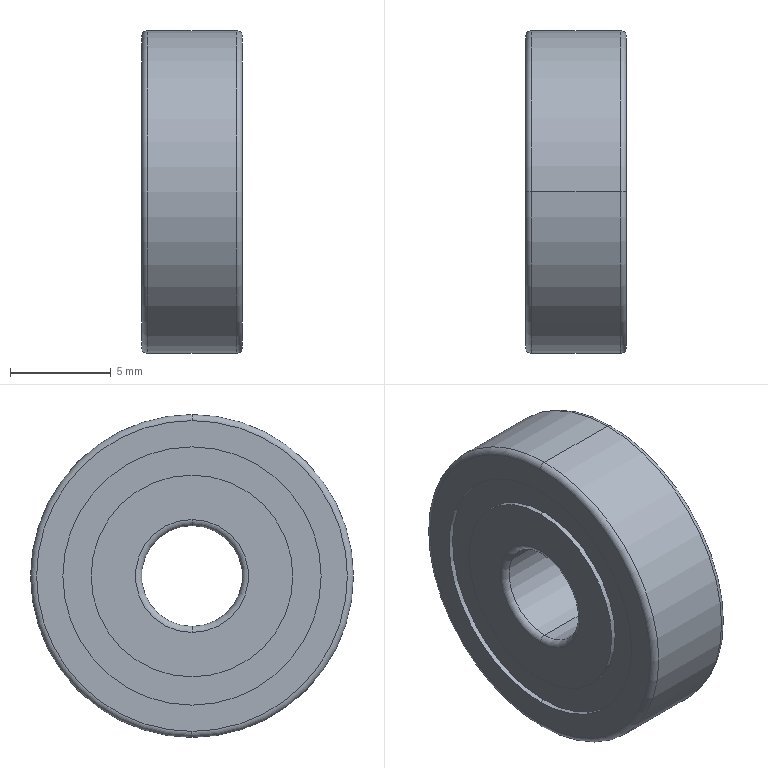Part | SolidWorks | features Revolution 1 | 1 solid | 26 faces | box 5 x 16 x 16 mm | volume 879.517 mm3 | cylinder 12 | torus 8 | plane 6 | commonest cylinder face diameters 10 x4 12.8 x4 5 x2 16 x2
STEP:
#1=CARTESIAN_POINT('',(2.2,0.,8.));
#2=VERTEX_POINT('',#1);
#3=CARTESIAN_POINT('',(2.2,0.,-8.));
#4=VERTEX_POINT('',#3);
#5=CARTESIAN_POINT('',(2.2,0.,0.));
#6=DIRECTION('',(-1.,0.,0.));
#7=DIRECTION('',(0.,0.,1.));
#8=AXIS2_PLACEMENT_3D('',#5,#6,#7);
#9=CIRCLE('',#8,8.);
#10=EDGE_CURVE('',#2,#4,#9,.T.);
#11=ORIENTED_EDGE('',*,*,#10,.T.);
#12=CARTESIAN_POINT('',(-2.2,0.,-8.));
#13=VERTEX_POINT('',#12);
#14=CARTESIAN_POINT('',(2.5,0.,-8.));
#15=DIRECTION('',(-1.,0.,0.));
#16=VECTOR('',#15,1000.);
#17=LINE('',#14,#16);
#18=EDGE_CURVE('',#4,#13,#17,.T.);
#19=ORIENTED_EDGE('',*,*,#18,.T.);
#20=CARTESIAN_POINT('',(-2.2,0.,8.));
#21=VERTEX_POINT('',#20);
#22=CARTESIAN_POINT('',(-2.2,0.,0.));
#23=DIRECTION('',(-1.,0.,0.));
#24=DIRECTION('',(0.,0.,1.));
#25=AXIS2_PLACEMENT_3D('',#22,#23,#24);
#26=CIRCLE('',#25,8.);
#27=EDGE_CURVE('',#21,#13,#26,.T.);
#28=ORIENTED_EDGE('',*,*,#27,.F.);
#29=CARTESIAN_POINT('',(2.5,0.,8.));
#30=DIRECTION('',(-1.,0.,0.));
#31=VECTOR('',#30,1000.);
#32=LINE('',#29,#31);
#33=EDGE_CURVE('',#2,#21,#32,.T.);
#34=ORIENTED_EDGE('',*,*,#33,.F.);
#35=EDGE_LOOP('',(#11,#19,#28,#34));
#36=FACE_OUTER_BOUND('',#35,.T.);
#37=CARTESIAN_POINT('',(2.5,0.,0.));
#38=DIRECTION('',(-1.,0.,0.));
#39=DIRECTION('',(0.,0.,1.));
#40=AXIS2_PLACEMENT_3D('',#37,#38,#39);
#41=CYLINDRICAL_SURFACE('',#40,8.);
#42=ADVANCED_FACE('',(#36),#41,.T.);
#43=CARTESIAN_POINT('',(2.5,0.,7.7));
#44=VERTEX_POINT('',#43);
#45=CARTESIAN_POINT('',(2.5,0.,-7.7));
#46=VERTEX_POINT('',#45);
#47=CARTESIAN_POINT('',(2.5,0.,0.));
#48=DIRECTION('',(-1.,0.,0.));
#49=DIRECTION('',(0.,0.,1.));
#50=AXIS2_PLACEMENT_3D('',#47,#48,#49);
#51=CIRCLE('',#50,7.7);
#52=EDGE_CURVE('',#44,#46,#51,.T.);
#53=ORIENTED_EDGE('',*,*,#52,.T.);
#54=CARTESIAN_POINT('',(2.2,0.,-7.7));
#55=DIRECTION('',(0.,1.,0.));
#56=DIRECTION('',(0.,0.,1.));
#57=AXIS2_PLACEMENT_3D('',#54,#55,#56);
#58=CIRCLE('',#57,0.3);
#59=EDGE_CURVE('',#46,#4,#58,.T.);
#60=ORIENTED_EDGE('',*,*,#59,.T.);
#61=ORIENTED_EDGE('',*,*,#10,.F.);
#62=CARTESIAN_POINT('',(2.2,0.,7.7));
#63=DIRECTION('',(0.,-1.,0.));
#64=DIRECTION('',(0.,0.,-1.));
#65=AXIS2_PLACEMENT_3D('',#62,#63,#64);
#66=CIRCLE('',#65,0.3);
#67=EDGE_CURVE('',#44,#2,#66,.T.);
#68=ORIENTED_EDGE('',*,*,#67,.F.);
#69=EDGE_LOOP('',(#53,#60,#61,#68));
#70=FACE_OUTER_BOUND('',#69,.T.);
#71=CARTESIAN_POINT('',(2.2,0.,0.));
#72=DIRECTION('',(-1.,0.,0.));
#73=DIRECTION('',(0.,0.,1.));
#74=AXIS2_PLACEMENT_3D('',#71,#72,#73);
#75=TOROIDAL_SURFACE('',#74,7.7,0.3);
#76=ADVANCED_FACE('',(#70),#75,.T.);
#77=CARTESIAN_POINT('',(2.5,0.,-6.4));
#78=VERTEX_POINT('',#77);
#79=CARTESIAN_POINT('',(2.5,0.,6.4));
#80=VERTEX_POINT('',#79);
#81=CARTESIAN_POINT('',(2.5,0.,0.));
#82=DIRECTION('',(-1.,0.,0.));
#83=DIRECTION('',(0.,0.,1.));
#84=AXIS2_PLACEMENT_3D('',#81,#82,#83);
#85=CIRCLE('',#84,6.4);
#86=EDGE_CURVE('',#78,#80,#85,.T.);
#87=ORIENTED_EDGE('',*,*,#86,.F.);
#88=CARTESIAN_POINT('',(2.25,0.,-6.4));
#89=VERTEX_POINT('',#88);
#90=CARTESIAN_POINT('',(2.5,0.,-6.4));
#91=DIRECTION('',(-1.,0.,0.));
#92=VECTOR('',#91,1000.);
#93=LINE('',#90,#92);
#94=EDGE_CURVE('',#78,#89,#93,.T.);
#95=ORIENTED_EDGE('',*,*,#94,.T.);
#96=CARTESIAN_POINT('',(2.25,0.,6.4));
#97=VERTEX_POINT('',#96);
#98=CARTESIAN_POINT('',(2.25,0.,0.));
#99=DIRECTION('',(-1.,0.,0.));
#100=DIRECTION('',(0.,0.,1.));
#101=AXIS2_PLACEMENT_3D('',#98,#99,#100);
#102=CIRCLE('',#101,6.4);
#103=EDGE_CURVE('',#89,#97,#102,.T.);
#104=ORIENTED_EDGE('',*,*,#103,.T.);
#105=CARTESIAN_POINT('',(2.5,0.,6.4));
#106=DIRECTION('',(-1.,0.,0.));
#107=VECTOR('',#106,1000.);
#108=LINE('',#105,#107);
#109=EDGE_CURVE('',#80,#97,#108,.T.);
#110=ORIENTED_EDGE('',*,*,#109,.F.);
#111=EDGE_LOOP('',(#87,#95,#104,#110));
#112=FACE_OUTER_BOUND('',#111,.T.);
#113=CARTESIAN_POINT('',(2.5,0.,0.));
#114=DIRECTION('',(-1.,0.,0.));
#115=DIRECTION('',(0.,0.,1.));
#116=AXIS2_PLACEMENT_3D('',#113,#114,#115);
#117=CYLINDRICAL_SURFACE('',#116,6.4);
#118=ADVANCED_FACE('',(#112),#117,.F.);
#119=CARTESIAN_POINT('',(2.5,0.,5.));
#120=VERTEX_POINT('',#119);
#121=CARTESIAN_POINT('',(2.5,0.,-5.));
#122=VERTEX_POINT('',#121);
#123=CARTESIAN_POINT('',(2.5,0.,0.));
#124=DIRECTION('',(-1.,0.,0.));
#125=DIRECTION('',(0.,0.,1.));
#126=AXIS2_PLACEMENT_3D('',#123,#124,#125);
#127=CIRCLE('',#126,5.);
#128=EDGE_CURVE('',#120,#122,#127,.T.);
#129=ORIENTED_EDGE('',*,*,#128,.T.);
#130=CARTESIAN_POINT('',(2.25,0.,-5.));
#131=VERTEX_POINT('',#130);
#132=CARTESIAN_POINT('',(2.5,0.,-5.));
#133=DIRECTION('',(-1.,0.,0.));
#134=VECTOR('',#133,1000.);
#135=LINE('',#132,#134);
#136=EDGE_CURVE('',#122,#131,#135,.T.);
#137=ORIENTED_EDGE('',*,*,#136,.T.);
#138=CARTESIAN_POINT('',(2.25,0.,5.));
#139=VERTEX_POINT('',#138);
#140=CARTESIAN_POINT('',(2.25,0.,0.));
#141=DIRECTION('',(-1.,0.,0.));
#142=DIRECTION('',(0.,0.,1.));
#143=AXIS2_PLACEMENT_3D('',#140,#141,#142);
#144=CIRCLE('',#143,5.);
#145=EDGE_CURVE('',#139,#131,#144,.T.);
#146=ORIENTED_EDGE('',*,*,#145,.F.);
#147=CARTESIAN_POINT('',(2.5,0.,5.));
#148=DIRECTION('',(-1.,0.,0.));
#149=VECTOR('',#148,1000.);
#150=LINE('',#147,#149);
#151=EDGE_CURVE('',#120,#139,#150,.T.);
#152=ORIENTED_EDGE('',*,*,#151,.F.);
#153=EDGE_LOOP('',(#129,#137,#146,#152));
#154=FACE_OUTER_BOUND('',#153,.T.);
#155=CARTESIAN_POINT('',(2.5,0.,0.));
#156=DIRECTION('',(-1.,0.,0.));
#157=DIRECTION('',(0.,0.,1.));
#158=AXIS2_PLACEMENT_3D('',#155,#156,#157);
#159=CYLINDRICAL_SURFACE('',#158,5.);
#160=ADVANCED_FACE('',(#154),#159,.T.);
#161=CARTESIAN_POINT('',(2.2,0.,2.5));
#162=VERTEX_POINT('',#161);
#163=CARTESIAN_POINT('',(2.2,0.,-2.5));
#164=VERTEX_POINT('',#163);
#165=CARTESIAN_POINT('',(2.2,0.,0.));
#166=DIRECTION('',(-1.,0.,0.));
#167=DIRECTION('',(0.,0.,1.));
#168=AXIS2_PLACEMENT_3D('',#165,#166,#167);
#169=CIRCLE('',#168,2.5);
#170=EDGE_CURVE('',#162,#164,#169,.T.);
#171=ORIENTED_EDGE('',*,*,#170,.T.);
#172=CARTESIAN_POINT('',(2.5,0.,-2.8));
#173=VERTEX_POINT('',#172);
#174=CARTESIAN_POINT('',(2.2,0.,-2.8));
#175=DIRECTION('',(0.,1.,0.));
#176=DIRECTION('',(0.,0.,1.));
#177=AXIS2_PLACEMENT_3D('',#174,#175,#176);
#178=CIRCLE('',#177,0.3);
#179=EDGE_CURVE('',#164,#173,#178,.T.);
#180=ORIENTED_EDGE('',*,*,#179,.T.);
#181=CARTESIAN_POINT('',(2.5,0.,2.8));
#182=VERTEX_POINT('',#181);
#183=CARTESIAN_POINT('',(2.5,0.,0.));
#184=DIRECTION('',(-1.,0.,0.));
#185=DIRECTION('',(0.,0.,1.));
#186=AXIS2_PLACEMENT_3D('',#183,#184,#185);
#187=CIRCLE('',#186,2.8);
#188=EDGE_CURVE('',#182,#173,#187,.T.);
#189=ORIENTED_EDGE('',*,*,#188,.F.);
#190=CARTESIAN_POINT('',(2.2,0.,2.8));
#191=DIRECTION('',(0.,-1.,0.));
#192=DIRECTION('',(0.,0.,-1.));
#193=AXIS2_PLACEMENT_3D('',#190,#191,#192);
#194=CIRCLE('',#193,0.3);
#195=EDGE_CURVE('',#162,#182,#194,.T.);
#196=ORIENTED_EDGE('',*,*,#195,.F.);
#197=EDGE_LOOP('',(#171,#180,#189,#196));
#198=FACE_OUTER_BOUND('',#197,.T.);
#199=CARTESIAN_POINT('',(2.2,0.,0.));
#200=DIRECTION('',(-1.,0.,0.));
#201=DIRECTION('',(0.,0.,1.));
#202=AXIS2_PLACEMENT_3D('',#199,#200,#201);
#203=TOROIDAL_SURFACE('',#202,2.8,0.3);
#204=ADVANCED_FACE('',(#198),#203,.T.);
#205=CARTESIAN_POINT('',(2.2,0.,0.));
#206=DIRECTION('',(-1.,0.,0.));
#207=DIRECTION('',(0.,0.,1.));
#208=AXIS2_PLACEMENT_3D('',#205,#206,#207);
#209=CIRCLE('',#208,2.5);
#210=EDGE_CURVE('',#164,#162,#209,.T.);
#211=ORIENTED_EDGE('',*,*,#210,.F.);
#212=CARTESIAN_POINT('',(-2.2,0.,-2.5));
#213=VERTEX_POINT('',#212);
#214=CARTESIAN_POINT('',(2.5,0.,-2.5));
#215=DIRECTION('',(-1.,0.,0.));
#216=VECTOR('',#215,1000.);
#217=LINE('',#214,#216);
#218=EDGE_CURVE('',#164,#213,#217,.T.);
#219=ORIENTED_EDGE('',*,*,#218,.T.);
#220=CARTESIAN_POINT('',(-2.2,0.,2.5));
#221=VERTEX_POINT('',#220);
#222=CARTESIAN_POINT('',(-2.2,0.,0.));
#223=DIRECTION('',(-1.,0.,0.));
#224=DIRECTION('',(0.,0.,1.));
#225=AXIS2_PLACEMENT_3D('',#222,#223,#224);
#226=CIRCLE('',#225,2.5);
#227=EDGE_CURVE('',#213,#221,#226,.T.);
#228=ORIENTED_EDGE('',*,*,#227,.T.);
#229=CARTESIAN_POINT('',(2.5,0.,2.5));
#230=DIRECTION('',(-1.,0.,0.));
#231=VECTOR('',#230,1000.);
#232=LINE('',#229,#231);
#233=EDGE_CURVE('',#162,#221,#232,.T.);
#234=ORIENTED_EDGE('',*,*,#233,.F.);
#235=EDGE_LOOP('',(#211,#219,#228,#234));
#236=FACE_OUTER_BOUND('',#235,.T.);
#237=CARTESIAN_POINT('',(2.5,0.,0.));
#238=DIRECTION('',(-1.,0.,0.));
#239=DIRECTION('',(0.,0.,1.));
#240=AXIS2_PLACEMENT_3D('',#237,#238,#239);
#241=CYLINDRICAL_SURFACE('',#240,2.5);
#242=ADVANCED_FACE('',(#236),#241,.F.);
#243=CARTESIAN_POINT('',(-2.5,0.,2.8));
#244=VERTEX_POINT('',#243);
#245=CARTESIAN_POINT('',(-2.5,0.,-2.8));
#246=VERTEX_POINT('',#245);
#247=CARTESIAN_POINT('',(-2.5,0.,0.));
#248=DIRECTION('',(-1.,0.,0.));
#249=DIRECTION('',(0.,0.,1.));
#250=AXIS2_PLACEMENT_3D('',#247,#248,#249);
#251=CIRCLE('',#250,2.8);
#252=EDGE_CURVE('',#244,#246,#251,.T.);
#253=ORIENTED_EDGE('',*,*,#252,.T.);
#254=CARTESIAN_POINT('',(-2.2,0.,-2.8));
#255=DIRECTION('',(0.,1.,0.));
#256=DIRECTION('',(0.,0.,1.));
#257=AXIS2_PLACEMENT_3D('',#254,#255,#256);
#258=CIRCLE('',#257,0.3);
#259=EDGE_CURVE('',#246,#213,#258,.T.);
#260=ORIENTED_EDGE('',*,*,#259,.T.);
#261=CARTESIAN_POINT('',(-2.2,0.,0.));
#262=DIRECTION('',(-1.,0.,0.));
#263=DIRECTION('',(0.,0.,1.));
#264=AXIS2_PLACEMENT_3D('',#261,#262,#263);
#265=CIRCLE('',#264,2.5);
#266=EDGE_CURVE('',#221,#213,#265,.T.);
#267=ORIENTED_EDGE('',*,*,#266,.F.);
#268=CARTESIAN_POINT('',(-2.2,0.,2.8));
#269=DIRECTION('',(0.,-1.,0.));
#270=DIRECTION('',(0.,0.,-1.));
#271=AXIS2_PLACEMENT_3D('',#268,#269,#270);
#272=CIRCLE('',#271,0.3);
#273=EDGE_CURVE('',#244,#221,#272,.T.);
#274=ORIENTED_EDGE('',*,*,#273,.F.);
#275=EDGE_LOOP('',(#253,#260,#267,#274));
#276=FACE_OUTER_BOUND('',#275,.T.);
#277=CARTESIAN_POINT('',(-2.2,0.,0.));
#278=DIRECTION('',(-1.,0.,0.));
#279=DIRECTION('',(0.,0.,1.));
#280=AXIS2_PLACEMENT_3D('',#277,#278,#279);
#281=TOROIDAL_SURFACE('',#280,2.8,0.3);
#282=ADVANCED_FACE('',(#276),#281,.T.);
#283=CARTESIAN_POINT('',(-2.25,0.,5.));
#284=VERTEX_POINT('',#283);
#285=CARTESIAN_POINT('',(-2.25,0.,-5.));
#286=VERTEX_POINT('',#285);
#287=CARTESIAN_POINT('',(-2.25,0.,0.));
#288=DIRECTION('',(-1.,0.,0.));
#289=DIRECTION('',(0.,0.,1.));
#290=AXIS2_PLACEMENT_3D('',#287,#288,#289);
#291=CIRCLE('',#290,5.);
#292=EDGE_CURVE('',#284,#286,#291,.T.);
#293=ORIENTED_EDGE('',*,*,#292,.T.);
#294=CARTESIAN_POINT('',(-2.5,0.,-5.));
#295=VERTEX_POINT('',#294);
#296=CARTESIAN_POINT('',(2.5,0.,-5.));
#297=DIRECTION('',(-1.,0.,0.));
#298=VECTOR('',#297,1000.);
#299=LINE('',#296,#298);
#300=EDGE_CURVE('',#286,#295,#299,.T.);
#301=ORIENTED_EDGE('',*,*,#300,.T.);
#302=CARTESIAN_POINT('',(-2.5,0.,5.));
#303=VERTEX_POINT('',#302);
#304=CARTESIAN_POINT('',(-2.5,0.,0.));
#305=DIRECTION('',(-1.,0.,0.));
#306=DIRECTION('',(0.,0.,1.));
#307=AXIS2_PLACEMENT_3D('',#304,#305,#306);
#308=CIRCLE('',#307,5.);
#309=EDGE_CURVE('',#303,#295,#308,.T.);
#310=ORIENTED_EDGE('',*,*,#309,.F.);
#311=CARTESIAN_POINT('',(2.5,0.,5.));
#312=DIRECTION('',(-1.,0.,0.));
#313=VECTOR('',#312,1000.);
#314=LINE('',#311,#313);
#315=EDGE_CURVE('',#284,#303,#314,.T.);
#316=ORIENTED_EDGE('',*,*,#315,.F.);
#317=EDGE_LOOP('',(#293,#301,#310,#316));
#318=FACE_OUTER_BOUND('',#317,.T.);
#319=CARTESIAN_POINT('',(2.5,0.,0.));
#320=DIRECTION('',(-1.,0.,0.));
#321=DIRECTION('',(0.,0.,1.));
#322=AXIS2_PLACEMENT_3D('',#319,#320,#321);
#323=CYLINDRICAL_SURFACE('',#322,5.);
#324=ADVANCED_FACE('',(#318),#323,.T.);
#325=CARTESIAN_POINT('',(-2.25,0.,-6.4));
#326=VERTEX_POINT('',#325);
#327=CARTESIAN_POINT('',(-2.25,0.,6.4));
#328=VERTEX_POINT('',#327);
#329=CARTESIAN_POINT('',(-2.25,0.,0.));
#330=DIRECTION('',(-1.,0.,0.));
#331=DIRECTION('',(0.,0.,1.));
#332=AXIS2_PLACEMENT_3D('',#329,#330,#331);
#333=CIRCLE('',#332,6.4);
#334=EDGE_CURVE('',#326,#328,#333,.T.);
#335=ORIENTED_EDGE('',*,*,#334,.F.);
#336=CARTESIAN_POINT('',(-2.5,0.,-6.4));
#337=VERTEX_POINT('',#336);
#338=CARTESIAN_POINT('',(2.5,0.,-6.4));
#339=DIRECTION('',(-1.,0.,0.));
#340=VECTOR('',#339,1000.);
#341=LINE('',#338,#340);
#342=EDGE_CURVE('',#326,#337,#341,.T.);
#343=ORIENTED_EDGE('',*,*,#342,.T.);
#344=CARTESIAN_POINT('',(-2.5,0.,6.4));
#345=VERTEX_POINT('',#344);
#346=CARTESIAN_POINT('',(-2.5,0.,0.));
#347=DIRECTION('',(-1.,0.,0.));
#348=DIRECTION('',(0.,0.,1.));
#349=AXIS2_PLACEMENT_3D('',#346,#347,#348);
#350=CIRCLE('',#349,6.4);
#351=EDGE_CURVE('',#337,#345,#350,.T.);
#352=ORIENTED_EDGE('',*,*,#351,.T.);
#353=CARTESIAN_POINT('',(2.5,0.,6.4));
#354=DIRECTION('',(-1.,0.,0.));
#355=VECTOR('',#354,1000.);
#356=LINE('',#353,#355);
#357=EDGE_CURVE('',#328,#345,#356,.T.);
#358=ORIENTED_EDGE('',*,*,#357,.F.);
#359=EDGE_LOOP('',(#335,#343,#352,#358));
#360=FACE_OUTER_BOUND('',#359,.T.);
#361=CARTESIAN_POINT('',(2.5,0.,0.));
#362=DIRECTION('',(-1.,0.,0.));
#363=DIRECTION('',(0.,0.,1.));
#364=AXIS2_PLACEMENT_3D('',#361,#362,#363);
#365=CYLINDRICAL_SURFACE('',#364,6.4);
#366=ADVANCED_FACE('',(#360),#365,.F.);
#367=ORIENTED_EDGE('',*,*,#27,.T.);
#368=CARTESIAN_POINT('',(-2.5,0.,-7.7));
#369=VERTEX_POINT('',#368);
#370=CARTESIAN_POINT('',(-2.2,0.,-7.7));
#371=DIRECTION('',(0.,1.,0.));
#372=DIRECTION('',(0.,0.,1.));
#373=AXIS2_PLACEMENT_3D('',#370,#371,#372);
#374=CIRCLE('',#373,0.3);
#375=EDGE_CURVE('',#13,#369,#374,.T.);
#376=ORIENTED_EDGE('',*,*,#375,.T.);
#377=CARTESIAN_POINT('',(-2.5,0.,7.7));
#378=VERTEX_POINT('',#377);
#379=CARTESIAN_POINT('',(-2.5,0.,0.));
#380=DIRECTION('',(-1.,0.,0.));
#381=DIRECTION('',(0.,0.,1.));
#382=AXIS2_PLACEMENT_3D('',#379,#380,#381);
#383=CIRCLE('',#382,7.7);
#384=EDGE_CURVE('',#378,#369,#383,.T.);
#385=ORIENTED_EDGE('',*,*,#384,.F.);
#386=CARTESIAN_POINT('',(-2.2,0.,7.7));
#387=DIRECTION('',(0.,-1.,0.));
#388=DIRECTION('',(0.,0.,-1.));
#389=AXIS2_PLACEMENT_3D('',#386,#387,#388);
#390=CIRCLE('',#389,0.3);
#391=EDGE_CURVE('',#21,#378,#390,.T.);
#392=ORIENTED_EDGE('',*,*,#391,.F.);
#393=EDGE_LOOP('',(#367,#376,#385,#392));
#394=FACE_OUTER_BOUND('',#393,.T.);
#395=CARTESIAN_POINT('',(-2.2,0.,0.));
#396=DIRECTION('',(-1.,0.,0.));
#397=DIRECTION('',(0.,0.,1.));
#398=AXIS2_PLACEMENT_3D('',#395,#396,#397);
#399=TOROIDAL_SURFACE('',#398,7.7,0.3);
#400=ADVANCED_FACE('',(#394),#399,.T.);
#401=ORIENTED_EDGE('',*,*,#375,.F.);
#402=CARTESIAN_POINT('',(-2.2,0.,0.));
#403=DIRECTION('',(-1.,0.,0.));
#404=DIRECTION('',(0.,0.,1.));
#405=AXIS2_PLACEMENT_3D('',#402,#403,#404);
#406=CIRCLE('',#405,8.);
#407=EDGE_CURVE('',#13,#21,#406,.T.);
#408=ORIENTED_EDGE('',*,*,#407,.T.);
#409=ORIENTED_EDGE('',*,*,#391,.T.);
#410=CARTESIAN_POINT('',(-2.5,0.,0.));
#411=DIRECTION('',(-1.,0.,0.));
#412=DIRECTION('',(0.,0.,1.));
#413=AXIS2_PLACEMENT_3D('',#410,#411,#412);
#414=CIRCLE('',#413,7.7);
#415=EDGE_CURVE('',#369,#378,#414,.T.);
#416=ORIENTED_EDGE('',*,*,#415,.F.);
#417=EDGE_LOOP('',(#401,#408,#409,#416));
#418=FACE_OUTER_BOUND('',#417,.T.);
#419=CARTESIAN_POINT('',(-2.2,0.,0.));
#420=DIRECTION('',(-1.,0.,0.));
#421=DIRECTION('',(0.,0.,1.));
#422=AXIS2_PLACEMENT_3D('',#419,#420,#421);
#423=TOROIDAL_SURFACE('',#422,7.7,0.3);
#424=ADVANCED_FACE('',(#418),#423,.T.);
#425=CARTESIAN_POINT('',(-2.5,0.,0.));
#426=DIRECTION('',(-1.,0.,0.));
#427=DIRECTION('',(0.,0.,1.));
#428=AXIS2_PLACEMENT_3D('',#425,#426,#427);
#429=CIRCLE('',#428,6.4);
#430=EDGE_CURVE('',#345,#337,#429,.T.);
#431=ORIENTED_EDGE('',*,*,#430,.F.);
#432=ORIENTED_EDGE('',*,*,#351,.F.);
#433=EDGE_LOOP('',(#431,#432));
#434=FACE_BOUND('',#433,.T.);
#435=ORIENTED_EDGE('',*,*,#384,.T.);
#436=ORIENTED_EDGE('',*,*,#415,.T.);
#437=EDGE_LOOP('',(#435,#436));
#438=FACE_OUTER_BOUND('',#437,.T.);
#439=CARTESIAN_POINT('',(-2.5,7.7,0.));
#440=DIRECTION('',(1.,0.,0.));
#441=DIRECTION('',(0.,0.,-1.));
#442=AXIS2_PLACEMENT_3D('',#439,#440,#441);
#443=PLANE('',#442);
#444=ADVANCED_FACE('',(#434,#438),#443,.F.);
#445=ORIENTED_EDGE('',*,*,#342,.F.);
#446=CARTESIAN_POINT('',(-2.25,0.,0.));
#447=DIRECTION('',(-1.,0.,0.));
#448=DIRECTION('',(0.,0.,1.));
#449=AXIS2_PLACEMENT_3D('',#446,#447,#448);
#450=CIRCLE('',#449,6.4);
#451=EDGE_CURVE('',#328,#326,#450,.T.);
#452=ORIENTED_EDGE('',*,*,#451,.F.);
#453=ORIENTED_EDGE('',*,*,#357,.T.);
#454=ORIENTED_EDGE('',*,*,#430,.T.);
#455=EDGE_LOOP('',(#445,#452,#453,#454));
#456=FACE_OUTER_BOUND('',#455,.T.);
#457=CARTESIAN_POINT('',(2.5,0.,0.));
#458=DIRECTION('',(-1.,0.,0.));
#459=DIRECTION('',(0.,0.,1.));
#460=AXIS2_PLACEMENT_3D('',#457,#458,#459);
#461=CYLINDRICAL_SURFACE('',#460,6.4);
#462=ADVANCED_FACE('',(#456),#461,.F.);
#463=ORIENTED_EDGE('',*,*,#292,.F.);
#464=CARTESIAN_POINT('',(-2.25,0.,0.));
#465=DIRECTION('',(-1.,0.,0.));
#466=DIRECTION('',(0.,0.,1.));
#467=AXIS2_PLACEMENT_3D('',#464,#465,#466);
#468=CIRCLE('',#467,5.);
#469=EDGE_CURVE('',#286,#284,#468,.T.);
#470=ORIENTED_EDGE('',*,*,#469,.F.);
#471=EDGE_LOOP('',(#463,#470));
#472=FACE_BOUND('',#471,.T.);
#473=ORIENTED_EDGE('',*,*,#451,.T.);
#474=ORIENTED_EDGE('',*,*,#334,.T.);
#475=EDGE_LOOP('',(#473,#474));
#476=FACE_OUTER_BOUND('',#475,.T.);
#477=CARTESIAN_POINT('',(-2.25,6.4,0.));
#478=DIRECTION('',(1.,0.,0.));
#479=DIRECTION('',(0.,0.,-1.));
#480=AXIS2_PLACEMENT_3D('',#477,#478,#479);
#481=PLANE('',#480);
#482=ADVANCED_FACE('',(#472,#476),#481,.F.);
#483=ORIENTED_EDGE('',*,*,#300,.F.);
#484=ORIENTED_EDGE('',*,*,#469,.T.);
#485=ORIENTED_EDGE('',*,*,#315,.T.);
#486=CARTESIAN_POINT('',(-2.5,0.,0.));
#487=DIRECTION('',(-1.,0.,0.));
#488=DIRECTION('',(0.,0.,1.));
#489=AXIS2_PLACEMENT_3D('',#486,#487,#488);
#490=CIRCLE('',#489,5.);
#491=EDGE_CURVE('',#295,#303,#490,.T.);
#492=ORIENTED_EDGE('',*,*,#491,.F.);
#493=EDGE_LOOP('',(#483,#484,#485,#492));
#494=FACE_OUTER_BOUND('',#493,.T.);
#495=CARTESIAN_POINT('',(2.5,0.,0.));
#496=DIRECTION('',(-1.,0.,0.));
#497=DIRECTION('',(0.,0.,1.));
#498=AXIS2_PLACEMENT_3D('',#495,#496,#497);
#499=CYLINDRICAL_SURFACE('',#498,5.);
#500=ADVANCED_FACE('',(#494),#499,.T.);
#501=ORIENTED_EDGE('',*,*,#252,.F.);
#502=CARTESIAN_POINT('',(-2.5,0.,0.));
#503=DIRECTION('',(-1.,0.,0.));
#504=DIRECTION('',(0.,0.,1.));
#505=AXIS2_PLACEMENT_3D('',#502,#503,#504);
#506=CIRCLE('',#505,2.8);
#507=EDGE_CURVE('',#246,#244,#506,.T.);
#508=ORIENTED_EDGE('',*,*,#507,.F.);
#509=EDGE_LOOP('',(#501,#508));
#510=FACE_BOUND('',#509,.T.);
#511=ORIENTED_EDGE('',*,*,#309,.T.);
#512=ORIENTED_EDGE('',*,*,#491,.T.);
#513=EDGE_LOOP('',(#511,#512));
#514=FACE_OUTER_BOUND('',#513,.T.);
#515=CARTESIAN_POINT('',(-2.5,5.,0.));
#516=DIRECTION('',(1.,0.,0.));
#517=DIRECTION('',(0.,0.,-1.));
#518=AXIS2_PLACEMENT_3D('',#515,#516,#517);
#519=PLANE('',#518);
#520=ADVANCED_FACE('',(#510,#514),#519,.F.);
#521=ORIENTED_EDGE('',*,*,#259,.F.);
#522=ORIENTED_EDGE('',*,*,#507,.T.);
#523=ORIENTED_EDGE('',*,*,#273,.T.);
#524=ORIENTED_EDGE('',*,*,#227,.F.);
#525=EDGE_LOOP('',(#521,#522,#523,#524));
#526=FACE_OUTER_BOUND('',#525,.T.);
#527=CARTESIAN_POINT('',(-2.2,0.,0.));
#528=DIRECTION('',(-1.,0.,0.));
#529=DIRECTION('',(0.,0.,1.));
#530=AXIS2_PLACEMENT_3D('',#527,#528,#529);
#531=TOROIDAL_SURFACE('',#530,2.8,0.3);
#532=ADVANCED_FACE('',(#526),#531,.T.);
#533=ORIENTED_EDGE('',*,*,#218,.F.);
#534=ORIENTED_EDGE('',*,*,#170,.F.);
#535=ORIENTED_EDGE('',*,*,#233,.T.);
#536=ORIENTED_EDGE('',*,*,#266,.T.);
#537=EDGE_LOOP('',(#533,#534,#535,#536));
#538=FACE_OUTER_BOUND('',#537,.T.);
#539=CARTESIAN_POINT('',(2.5,0.,0.));
#540=DIRECTION('',(-1.,0.,0.));
#541=DIRECTION('',(0.,0.,1.));
#542=AXIS2_PLACEMENT_3D('',#539,#540,#541);
#543=CYLINDRICAL_SURFACE('',#542,2.5);
#544=ADVANCED_FACE('',(#538),#543,.F.);
#545=ORIENTED_EDGE('',*,*,#179,.F.);
#546=ORIENTED_EDGE('',*,*,#210,.T.);
#547=ORIENTED_EDGE('',*,*,#195,.T.);
#548=CARTESIAN_POINT('',(2.5,0.,0.));
#549=DIRECTION('',(-1.,0.,0.));
#550=DIRECTION('',(0.,0.,1.));
#551=AXIS2_PLACEMENT_3D('',#548,#549,#550);
#552=CIRCLE('',#551,2.8);
#553=EDGE_CURVE('',#173,#182,#552,.T.);
#554=ORIENTED_EDGE('',*,*,#553,.F.);
#555=EDGE_LOOP('',(#545,#546,#547,#554));
#556=FACE_OUTER_BOUND('',#555,.T.);
#557=CARTESIAN_POINT('',(2.2,0.,0.));
#558=DIRECTION('',(-1.,0.,0.));
#559=DIRECTION('',(0.,0.,1.));
#560=AXIS2_PLACEMENT_3D('',#557,#558,#559);
#561=TOROIDAL_SURFACE('',#560,2.8,0.3);
#562=ADVANCED_FACE('',(#556),#561,.T.);
#563=ORIENTED_EDGE('',*,*,#128,.F.);
#564=CARTESIAN_POINT('',(2.5,0.,0.));
#565=DIRECTION('',(-1.,0.,0.));
#566=DIRECTION('',(0.,0.,1.));
#567=AXIS2_PLACEMENT_3D('',#564,#565,#566);
#568=CIRCLE('',#567,5.);
#569=EDGE_CURVE('',#122,#120,#568,.T.);
#570=ORIENTED_EDGE('',*,*,#569,.F.);
#571=EDGE_LOOP('',(#563,#570));
#572=FACE_OUTER_BOUND('',#571,.T.);
#573=ORIENTED_EDGE('',*,*,#188,.T.);
#574=ORIENTED_EDGE('',*,*,#553,.T.);
#575=EDGE_LOOP('',(#573,#574));
#576=FACE_BOUND('',#575,.T.);
#577=CARTESIAN_POINT('',(2.5,2.8,0.));
#578=DIRECTION('',(-1.,0.,0.));
#579=DIRECTION('',(0.,0.,1.));
#580=AXIS2_PLACEMENT_3D('',#577,#578,#579);
#581=PLANE('',#580);
#582=ADVANCED_FACE('',(#572,#576),#581,.F.);
#583=ORIENTED_EDGE('',*,*,#136,.F.);
#584=ORIENTED_EDGE('',*,*,#569,.T.);
#585=ORIENTED_EDGE('',*,*,#151,.T.);
#586=CARTESIAN_POINT('',(2.25,0.,0.));
#587=DIRECTION('',(-1.,0.,0.));
#588=DIRECTION('',(0.,0.,1.));
#589=AXIS2_PLACEMENT_3D('',#586,#587,#588);
#590=CIRCLE('',#589,5.);
#591=EDGE_CURVE('',#131,#139,#590,.T.);
#592=ORIENTED_EDGE('',*,*,#591,.F.);
#593=EDGE_LOOP('',(#583,#584,#585,#592));
#594=FACE_OUTER_BOUND('',#593,.T.);
#595=CARTESIAN_POINT('',(2.5,0.,0.));
#596=DIRECTION('',(-1.,0.,0.));
#597=DIRECTION('',(0.,0.,1.));
#598=AXIS2_PLACEMENT_3D('',#595,#596,#597);
#599=CYLINDRICAL_SURFACE('',#598,5.);
#600=ADVANCED_FACE('',(#594),#599,.T.);
#601=CARTESIAN_POINT('',(2.25,0.,0.));
#602=DIRECTION('',(-1.,0.,0.));
#603=DIRECTION('',(0.,0.,1.));
#604=AXIS2_PLACEMENT_3D('',#601,#602,#603);
#605=CIRCLE('',#604,6.4);
#606=EDGE_CURVE('',#97,#89,#605,.T.);
#607=ORIENTED_EDGE('',*,*,#606,.F.);
#608=ORIENTED_EDGE('',*,*,#103,.F.);
#609=EDGE_LOOP('',(#607,#608));
#610=FACE_OUTER_BOUND('',#609,.T.);
#611=ORIENTED_EDGE('',*,*,#145,.T.);
#612=ORIENTED_EDGE('',*,*,#591,.T.);
#613=EDGE_LOOP('',(#611,#612));
#614=FACE_BOUND('',#613,.T.);
#615=CARTESIAN_POINT('',(2.25,5.,0.));
#616=DIRECTION('',(-1.,0.,0.));
#617=DIRECTION('',(0.,0.,1.));
#618=AXIS2_PLACEMENT_3D('',#615,#616,#617);
#619=PLANE('',#618);
#620=ADVANCED_FACE('',(#610,#614),#619,.F.);
#621=ORIENTED_EDGE('',*,*,#94,.F.);
#622=CARTESIAN_POINT('',(2.5,0.,0.));
#623=DIRECTION('',(-1.,0.,0.));
#624=DIRECTION('',(0.,0.,1.));
#625=AXIS2_PLACEMENT_3D('',#622,#623,#624);
#626=CIRCLE('',#625,6.4);
#627=EDGE_CURVE('',#80,#78,#626,.T.);
#628=ORIENTED_EDGE('',*,*,#627,.F.);
#629=ORIENTED_EDGE('',*,*,#109,.T.);
#630=ORIENTED_EDGE('',*,*,#606,.T.);
#631=EDGE_LOOP('',(#621,#628,#629,#630));
#632=FACE_OUTER_BOUND('',#631,.T.);
#633=CARTESIAN_POINT('',(2.5,0.,0.));
#634=DIRECTION('',(-1.,0.,0.));
#635=DIRECTION('',(0.,0.,1.));
#636=AXIS2_PLACEMENT_3D('',#633,#634,#635);
#637=CYLINDRICAL_SURFACE('',#636,6.4);
#638=ADVANCED_FACE('',(#632),#637,.F.);
#639=ORIENTED_EDGE('',*,*,#52,.F.);
#640=CARTESIAN_POINT('',(2.5,0.,0.));
#641=DIRECTION('',(-1.,0.,0.));
#642=DIRECTION('',(0.,0.,1.));
#643=AXIS2_PLACEMENT_3D('',#640,#641,#642);
#644=CIRCLE('',#643,7.7);
#645=EDGE_CURVE('',#46,#44,#644,.T.);
#646=ORIENTED_EDGE('',*,*,#645,.F.);
#647=EDGE_LOOP('',(#639,#646));
#648=FACE_OUTER_BOUND('',#647,.T.);
#649=ORIENTED_EDGE('',*,*,#627,.T.);
#650=ORIENTED_EDGE('',*,*,#86,.T.);
#651=EDGE_LOOP('',(#649,#650));
#652=FACE_BOUND('',#651,.T.);
#653=CARTESIAN_POINT('',(2.5,6.4,0.));
#654=DIRECTION('',(-1.,0.,0.));
#655=DIRECTION('',(0.,0.,1.));
#656=AXIS2_PLACEMENT_3D('',#653,#654,#655);
#657=PLANE('',#656);
#658=ADVANCED_FACE('',(#648,#652),#657,.F.);
#659=ORIENTED_EDGE('',*,*,#59,.F.);
#660=ORIENTED_EDGE('',*,*,#645,.T.);
#661=ORIENTED_EDGE('',*,*,#67,.T.);
#662=CARTESIAN_POINT('',(2.2,0.,0.));
#663=DIRECTION('',(-1.,0.,0.));
#664=DIRECTION('',(0.,0.,1.));
#665=AXIS2_PLACEMENT_3D('',#662,#663,#664);
#666=CIRCLE('',#665,8.);
#667=EDGE_CURVE('',#4,#2,#666,.T.);
#668=ORIENTED_EDGE('',*,*,#667,.F.);
#669=EDGE_LOOP('',(#659,#660,#661,#668));
#670=FACE_OUTER_BOUND('',#669,.T.);
#671=CARTESIAN_POINT('',(2.2,0.,0.));
#672=DIRECTION('',(-1.,0.,0.));
#673=DIRECTION('',(0.,0.,1.));
#674=AXIS2_PLACEMENT_3D('',#671,#672,#673);
#675=TOROIDAL_SURFACE('',#674,7.7,0.3);
#676=ADVANCED_FACE('',(#670),#675,.T.);
#677=ORIENTED_EDGE('',*,*,#18,.F.);
#678=ORIENTED_EDGE('',*,*,#667,.T.);
#679=ORIENTED_EDGE('',*,*,#33,.T.);
#680=ORIENTED_EDGE('',*,*,#407,.F.);
#681=EDGE_LOOP('',(#677,#678,#679,#680));
#682=FACE_OUTER_BOUND('',#681,.T.);
#683=CARTESIAN_POINT('',(2.5,0.,0.));
#684=DIRECTION('',(-1.,0.,0.));
#685=DIRECTION('',(0.,0.,1.));
#686=AXIS2_PLACEMENT_3D('',#683,#684,#685);
#687=CYLINDRICAL_SURFACE('',#686,8.);
#688=ADVANCED_FACE('',(#682),#687,.T.);
#689=CLOSED_SHELL('',(#42,#76,#118,#160,#204,#242,#282,#324,#366,#400,#424,#444,#462,#482,#500,#520,#532,#544,#562,#582,#600,#620,#638,#658,#676,#688));
#690=MANIFOLD_SOLID_BREP('',#689);
#691=CARTESIAN_POINT('',(0.,0.,0.));
#692=DIRECTION('',(0.,0.,1.));
#693=DIRECTION('',(1.,0.,0.));
#694=AXIS2_PLACEMENT_3D('',#691,#692,#693);
#695=(LENGTH_UNIT()NAMED_UNIT(*)SI_UNIT(.MILLI.,.METRE.));
#696=UNCERTAINTY_MEASURE_WITH_UNIT(LENGTH_MEASURE(0.00001),#695,'','');
#697=(NAMED_UNIT(*)PLANE_ANGLE_UNIT()SI_UNIT($,.RADIAN.));
#698=(NAMED_UNIT(*)SI_UNIT($,.STERADIAN.)SOLID_ANGLE_UNIT());
#699=(GEOMETRIC_REPRESENTATION_CONTEXT(3)GLOBAL_UNCERTAINTY_ASSIGNED_CONTEXT((#696))GLOBAL_UNIT_ASSIGNED_CONTEXT((#695,#697,#698))REPRESENTATION_CONTEXT('',''));
#700=ADVANCED_BREP_SHAPE_REPRESENTATION('',(#690,#694),#699);